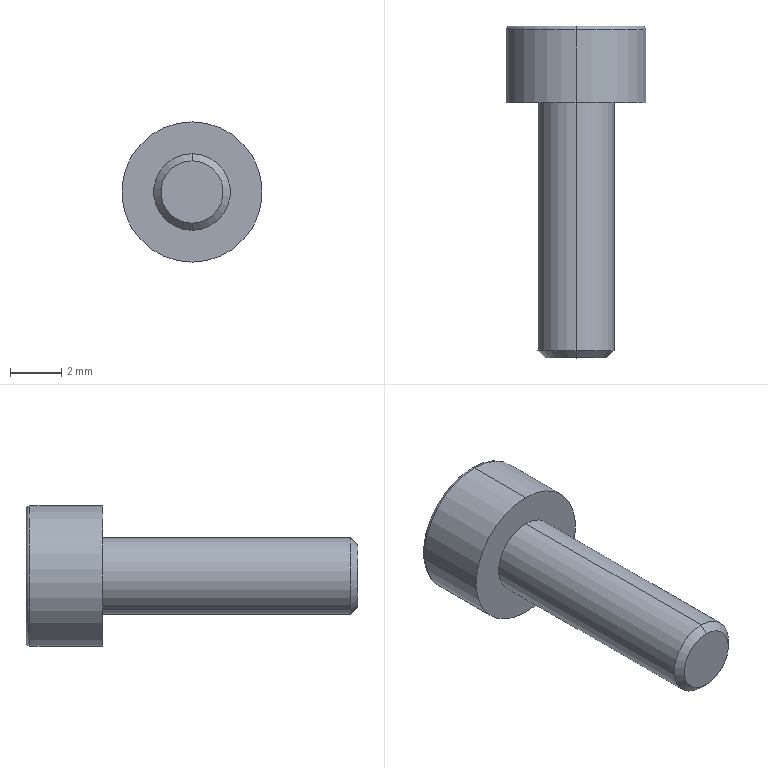Part | SolidWorks | features ICE 2, Chamfer 1, Extrusion 1, Fillet 1, RefAxis 1 | 1 solid | 18 faces | box 5.5 x 13 x 5.5 mm | volume 134.154 mm3 | plane 10 | cylinder 4 | cone 2 | torus 2 | commonest cylinder face diameters 3 x2 5.5 x2
STEP:
#1=CARTESIAN_POINT('',(0.,-10.,-1.22));
#2=VERTEX_POINT('',#1);
#3=CARTESIAN_POINT('',(0.,-10.,1.22));
#4=VERTEX_POINT('',#3);
#5=CARTESIAN_POINT('',(0.,-10.,0.));
#6=DIRECTION('',(0.,-1.,0.));
#7=DIRECTION('',(0.,0.,-1.));
#8=AXIS2_PLACEMENT_3D('',#5,#6,#7);
#9=CIRCLE('',#8,1.22);
#10=EDGE_CURVE('',#2,#4,#9,.T.);
#11=ORIENTED_EDGE('',*,*,#10,.F.);
#12=CARTESIAN_POINT('',(0.,-9.72,-1.5));
#13=VERTEX_POINT('',#12);
#14=CARTESIAN_POINT('',(0.,-10.,-1.22));
#15=DIRECTION('',(0.,0.7071,-0.7071));
#16=VECTOR('',#15,1000.);
#17=LINE('',#14,#16);
#18=EDGE_CURVE('',#2,#13,#17,.T.);
#19=ORIENTED_EDGE('',*,*,#18,.T.);
#20=CARTESIAN_POINT('',(0.,-9.72,1.5));
#21=VERTEX_POINT('',#20);
#22=CARTESIAN_POINT('',(0.,-9.72,0.));
#23=DIRECTION('',(0.,1.,0.));
#24=DIRECTION('',(0.,0.,-1.));
#25=AXIS2_PLACEMENT_3D('',#22,#23,#24);
#26=CIRCLE('',#25,1.5);
#27=EDGE_CURVE('',#21,#13,#26,.T.);
#28=ORIENTED_EDGE('',*,*,#27,.F.);
#29=CARTESIAN_POINT('',(0.,-10.,1.22));
#30=DIRECTION('',(0.,0.7071,0.7071));
#31=VECTOR('',#30,1000.);
#32=LINE('',#29,#31);
#33=EDGE_CURVE('',#4,#21,#32,.T.);
#34=ORIENTED_EDGE('',*,*,#33,.F.);
#35=EDGE_LOOP('',(#11,#19,#28,#34));
#36=FACE_OUTER_BOUND('',#35,.T.);
#37=CARTESIAN_POINT('',(0.,-10.,0.));
#38=DIRECTION('',(0.,1.,0.));
#39=DIRECTION('',(0.,0.,1.));
#40=AXIS2_PLACEMENT_3D('',#37,#38,#39);
#41=CONICAL_SURFACE('',#40,1.22,0.7854);
#42=ADVANCED_FACE('',(#36),#41,.T.);
#43=ORIENTED_EDGE('',*,*,#27,.T.);
#44=CARTESIAN_POINT('',(0.,0.,-1.5));
#45=VERTEX_POINT('',#44);
#46=CARTESIAN_POINT('',(0.,-10.,-1.5));
#47=DIRECTION('',(0.,1.,0.));
#48=VECTOR('',#47,1000.);
#49=LINE('',#46,#48);
#50=EDGE_CURVE('',#13,#45,#49,.T.);
#51=ORIENTED_EDGE('',*,*,#50,.T.);
#52=CARTESIAN_POINT('',(0.,0.,1.5));
#53=VERTEX_POINT('',#52);
#54=CARTESIAN_POINT('',(0.,0.,0.));
#55=DIRECTION('',(0.,-1.,0.));
#56=DIRECTION('',(0.,0.,1.));
#57=AXIS2_PLACEMENT_3D('',#54,#55,#56);
#58=CIRCLE('',#57,1.5);
#59=EDGE_CURVE('',#45,#53,#58,.T.);
#60=ORIENTED_EDGE('',*,*,#59,.T.);
#61=CARTESIAN_POINT('',(0.,-10.,1.5));
#62=DIRECTION('',(0.,1.,0.));
#63=VECTOR('',#62,1000.);
#64=LINE('',#61,#63);
#65=EDGE_CURVE('',#21,#53,#64,.T.);
#66=ORIENTED_EDGE('',*,*,#65,.F.);
#67=EDGE_LOOP('',(#43,#51,#60,#66));
#68=FACE_OUTER_BOUND('',#67,.T.);
#69=CARTESIAN_POINT('',(0.,-10.,0.));
#70=DIRECTION('',(0.,1.,0.));
#71=DIRECTION('',(0.,0.,1.));
#72=AXIS2_PLACEMENT_3D('',#69,#70,#71);
#73=CYLINDRICAL_SURFACE('',#72,1.5);
#74=ADVANCED_FACE('',(#68),#73,.T.);
#75=CARTESIAN_POINT('',(0.,2.85,-2.75));
#76=VERTEX_POINT('',#75);
#77=CARTESIAN_POINT('',(0.,2.85,2.75));
#78=VERTEX_POINT('',#77);
#79=CARTESIAN_POINT('',(0.,2.85,0.));
#80=DIRECTION('',(0.,-1.,0.));
#81=DIRECTION('',(0.,0.,1.));
#82=AXIS2_PLACEMENT_3D('',#79,#80,#81);
#83=CIRCLE('',#82,2.75);
#84=EDGE_CURVE('',#76,#78,#83,.T.);
#85=ORIENTED_EDGE('',*,*,#84,.F.);
#86=CARTESIAN_POINT('',(0.,3.,-2.6));
#87=VERTEX_POINT('',#86);
#88=CARTESIAN_POINT('',(0.,2.85,-2.6));
#89=DIRECTION('',(1.,0.,0.));
#90=DIRECTION('',(0.,0.,-1.));
#91=AXIS2_PLACEMENT_3D('',#88,#89,#90);
#92=CIRCLE('',#91,0.15);
#93=EDGE_CURVE('',#76,#87,#92,.T.);
#94=ORIENTED_EDGE('',*,*,#93,.T.);
#95=CARTESIAN_POINT('',(0.,3.,2.6));
#96=VERTEX_POINT('',#95);
#97=CARTESIAN_POINT('',(0.,3.,0.));
#98=DIRECTION('',(0.,1.,0.));
#99=DIRECTION('',(0.,0.,1.));
#100=AXIS2_PLACEMENT_3D('',#97,#98,#99);
#101=CIRCLE('',#100,2.6);
#102=EDGE_CURVE('',#96,#87,#101,.T.);
#103=ORIENTED_EDGE('',*,*,#102,.F.);
#104=CARTESIAN_POINT('',(0.,2.85,2.6));
#105=DIRECTION('',(-1.,0.,0.));
#106=DIRECTION('',(0.,0.,1.));
#107=AXIS2_PLACEMENT_3D('',#104,#105,#106);
#108=CIRCLE('',#107,0.15);
#109=EDGE_CURVE('',#78,#96,#108,.T.);
#110=ORIENTED_EDGE('',*,*,#109,.F.);
#111=EDGE_LOOP('',(#85,#94,#103,#110));
#112=FACE_OUTER_BOUND('',#111,.T.);
#113=CARTESIAN_POINT('',(0.,2.85,0.));
#114=DIRECTION('',(0.,1.,0.));
#115=DIRECTION('',(0.,0.,1.));
#116=AXIS2_PLACEMENT_3D('',#113,#114,#115);
#117=TOROIDAL_SURFACE('',#116,2.6,0.15);
#118=ADVANCED_FACE('',(#112),#117,.T.);
#119=ORIENTED_EDGE('',*,*,#84,.T.);
#120=CARTESIAN_POINT('',(0.,0.,2.75));
#121=VERTEX_POINT('',#120);
#122=CARTESIAN_POINT('',(0.,3.,2.75));
#123=DIRECTION('',(0.,-1.,0.));
#124=VECTOR('',#123,1000.);
#125=LINE('',#122,#124);
#126=EDGE_CURVE('',#78,#121,#125,.T.);
#127=ORIENTED_EDGE('',*,*,#126,.T.);
#128=CARTESIAN_POINT('',(0.,0.,-2.75));
#129=VERTEX_POINT('',#128);
#130=CARTESIAN_POINT('',(0.,0.,0.));
#131=DIRECTION('',(0.,1.,0.));
#132=DIRECTION('',(0.,0.,1.));
#133=AXIS2_PLACEMENT_3D('',#130,#131,#132);
#134=CIRCLE('',#133,2.75);
#135=EDGE_CURVE('',#121,#129,#134,.T.);
#136=ORIENTED_EDGE('',*,*,#135,.T.);
#137=CARTESIAN_POINT('',(0.,3.,-2.75));
#138=DIRECTION('',(0.,-1.,0.));
#139=VECTOR('',#138,1000.);
#140=LINE('',#137,#139);
#141=EDGE_CURVE('',#76,#129,#140,.T.);
#142=ORIENTED_EDGE('',*,*,#141,.F.);
#143=EDGE_LOOP('',(#119,#127,#136,#142));
#144=FACE_OUTER_BOUND('',#143,.T.);
#145=CARTESIAN_POINT('',(0.,3.,0.));
#146=DIRECTION('',(0.,-1.,0.));
#147=DIRECTION('',(0.,0.,-1.));
#148=AXIS2_PLACEMENT_3D('',#145,#146,#147);
#149=CYLINDRICAL_SURFACE('',#148,2.75);
#150=ADVANCED_FACE('',(#144),#149,.T.);
#151=CARTESIAN_POINT('',(0.,0.,0.));
#152=DIRECTION('',(0.,1.,0.));
#153=DIRECTION('',(0.,0.,1.));
#154=AXIS2_PLACEMENT_3D('',#151,#152,#153);
#155=CIRCLE('',#154,2.75);
#156=EDGE_CURVE('',#129,#121,#155,.T.);
#157=ORIENTED_EDGE('',*,*,#156,.F.);
#158=ORIENTED_EDGE('',*,*,#135,.F.);
#159=EDGE_LOOP('',(#157,#158));
#160=FACE_OUTER_BOUND('',#159,.T.);
#161=CARTESIAN_POINT('',(0.,0.,0.));
#162=DIRECTION('',(0.,-1.,0.));
#163=DIRECTION('',(0.,0.,1.));
#164=AXIS2_PLACEMENT_3D('',#161,#162,#163);
#165=CIRCLE('',#164,1.5);
#166=EDGE_CURVE('',#53,#45,#165,.T.);
#167=ORIENTED_EDGE('',*,*,#166,.F.);
#168=ORIENTED_EDGE('',*,*,#59,.F.);
#169=EDGE_LOOP('',(#167,#168));
#170=FACE_BOUND('',#169,.T.);
#171=CARTESIAN_POINT('',(0.,0.,0.));
#172=DIRECTION('',(0.,1.,0.));
#173=DIRECTION('',(0.,0.,1.));
#174=AXIS2_PLACEMENT_3D('',#171,#172,#173);
#175=PLANE('',#174);
#176=ADVANCED_FACE('',(#160,#170),#175,.F.);
#177=ORIENTED_EDGE('',*,*,#126,.F.);
#178=CARTESIAN_POINT('',(0.,2.85,0.));
#179=DIRECTION('',(0.,-1.,0.));
#180=DIRECTION('',(0.,0.,1.));
#181=AXIS2_PLACEMENT_3D('',#178,#179,#180);
#182=CIRCLE('',#181,2.75);
#183=EDGE_CURVE('',#78,#76,#182,.T.);
#184=ORIENTED_EDGE('',*,*,#183,.T.);
#185=ORIENTED_EDGE('',*,*,#141,.T.);
#186=ORIENTED_EDGE('',*,*,#156,.T.);
#187=EDGE_LOOP('',(#177,#184,#185,#186));
#188=FACE_OUTER_BOUND('',#187,.T.);
#189=CARTESIAN_POINT('',(0.,3.,0.));
#190=DIRECTION('',(0.,-1.,0.));
#191=DIRECTION('',(0.,0.,-1.));
#192=AXIS2_PLACEMENT_3D('',#189,#190,#191);
#193=CYLINDRICAL_SURFACE('',#192,2.75);
#194=ADVANCED_FACE('',(#188),#193,.T.);
#195=ORIENTED_EDGE('',*,*,#102,.T.);
#196=CARTESIAN_POINT('',(0.,3.,0.));
#197=DIRECTION('',(0.,1.,0.));
#198=DIRECTION('',(0.,0.,1.));
#199=AXIS2_PLACEMENT_3D('',#196,#197,#198);
#200=CIRCLE('',#199,2.6);
#201=EDGE_CURVE('',#87,#96,#200,.T.);
#202=ORIENTED_EDGE('',*,*,#201,.T.);
#203=EDGE_LOOP('',(#195,#202));
#204=FACE_OUTER_BOUND('',#203,.T.);
#205=CARTESIAN_POINT('',(0.739,3.,1.28));
#206=VERTEX_POINT('',#205);
#207=CARTESIAN_POINT('',(1.478,3.,0.));
#208=VERTEX_POINT('',#207);
#209=CARTESIAN_POINT('',(0.739,3.,1.28));
#210=DIRECTION('',(0.5,0.,-0.866));
#211=VECTOR('',#210,1000.);
#212=LINE('',#209,#211);
#213=EDGE_CURVE('',#206,#208,#212,.T.);
#214=ORIENTED_EDGE('',*,*,#213,.F.);
#215=CARTESIAN_POINT('',(-0.739,3.,1.28));
#216=VERTEX_POINT('',#215);
#217=CARTESIAN_POINT('',(-0.739,3.,1.28));
#218=DIRECTION('',(1.,0.,0.));
#219=VECTOR('',#218,1000.);
#220=LINE('',#217,#219);
#221=EDGE_CURVE('',#216,#206,#220,.T.);
#222=ORIENTED_EDGE('',*,*,#221,.F.);
#223=CARTESIAN_POINT('',(-1.478,3.,0.));
#224=VERTEX_POINT('',#223);
#225=CARTESIAN_POINT('',(-1.478,3.,0.));
#226=DIRECTION('',(0.5,0.,0.866));
#227=VECTOR('',#226,1000.);
#228=LINE('',#225,#227);
#229=EDGE_CURVE('',#224,#216,#228,.T.);
#230=ORIENTED_EDGE('',*,*,#229,.F.);
#231=CARTESIAN_POINT('',(-0.739,3.,-1.28));
#232=VERTEX_POINT('',#231);
#233=CARTESIAN_POINT('',(-0.739,3.,-1.28));
#234=DIRECTION('',(-0.5,0.,0.866));
#235=VECTOR('',#234,1000.);
#236=LINE('',#233,#235);
#237=EDGE_CURVE('',#232,#224,#236,.T.);
#238=ORIENTED_EDGE('',*,*,#237,.F.);
#239=CARTESIAN_POINT('',(0.739,3.,-1.28));
#240=VERTEX_POINT('',#239);
#241=CARTESIAN_POINT('',(0.739,3.,-1.28));
#242=DIRECTION('',(-1.,0.,0.));
#243=VECTOR('',#242,1000.);
#244=LINE('',#241,#243);
#245=EDGE_CURVE('',#240,#232,#244,.T.);
#246=ORIENTED_EDGE('',*,*,#245,.F.);
#247=CARTESIAN_POINT('',(1.478,3.,0.));
#248=DIRECTION('',(-0.5,0.,-0.866));
#249=VECTOR('',#248,1000.);
#250=LINE('',#247,#249);
#251=EDGE_CURVE('',#208,#240,#250,.T.);
#252=ORIENTED_EDGE('',*,*,#251,.F.);
#253=EDGE_LOOP('',(#214,#222,#230,#238,#246,#252));
#254=FACE_BOUND('',#253,.T.);
#255=CARTESIAN_POINT('',(0.,3.,0.));
#256=DIRECTION('',(0.,1.,0.));
#257=DIRECTION('',(0.,0.,1.));
#258=AXIS2_PLACEMENT_3D('',#255,#256,#257);
#259=PLANE('',#258);
#260=ADVANCED_FACE('',(#204,#254),#259,.T.);
#261=ORIENTED_EDGE('',*,*,#213,.T.);
#262=CARTESIAN_POINT('',(1.478,1.7,0.));
#263=VERTEX_POINT('',#262);
#264=CARTESIAN_POINT('',(1.478,1.7,0.));
#265=DIRECTION('',(0.,1.,0.));
#266=VECTOR('',#265,1000.);
#267=LINE('',#264,#266);
#268=EDGE_CURVE('',#263,#208,#267,.T.);
#269=ORIENTED_EDGE('',*,*,#268,.F.);
#270=CARTESIAN_POINT('',(0.739,1.7,1.28));
#271=VERTEX_POINT('',#270);
#272=CARTESIAN_POINT('',(0.739,1.7,1.28));
#273=DIRECTION('',(0.5,0.,-0.866));
#274=VECTOR('',#273,1000.);
#275=LINE('',#272,#274);
#276=EDGE_CURVE('',#271,#263,#275,.T.);
#277=ORIENTED_EDGE('',*,*,#276,.F.);
#278=CARTESIAN_POINT('',(0.739,1.7,1.28));
#279=DIRECTION('',(0.,1.,0.));
#280=VECTOR('',#279,1000.);
#281=LINE('',#278,#280);
#282=EDGE_CURVE('',#271,#206,#281,.T.);
#283=ORIENTED_EDGE('',*,*,#282,.T.);
#284=EDGE_LOOP('',(#261,#269,#277,#283));
#285=FACE_OUTER_BOUND('',#284,.T.);
#286=CARTESIAN_POINT('',(0.739,1.7,1.28));
#287=DIRECTION('',(0.866,0.,0.5));
#288=DIRECTION('',(0.5,0.,-0.866));
#289=AXIS2_PLACEMENT_3D('',#286,#287,#288);
#290=PLANE('',#289);
#291=ADVANCED_FACE('',(#285),#290,.F.);
#292=ORIENTED_EDGE('',*,*,#221,.T.);
#293=ORIENTED_EDGE('',*,*,#282,.F.);
#294=CARTESIAN_POINT('',(-0.739,1.7,1.28));
#295=VERTEX_POINT('',#294);
#296=CARTESIAN_POINT('',(-0.739,1.7,1.28));
#297=DIRECTION('',(1.,0.,0.));
#298=VECTOR('',#297,1000.);
#299=LINE('',#296,#298);
#300=EDGE_CURVE('',#295,#271,#299,.T.);
#301=ORIENTED_EDGE('',*,*,#300,.F.);
#302=CARTESIAN_POINT('',(-0.739,1.7,1.28));
#303=DIRECTION('',(0.,1.,0.));
#304=VECTOR('',#303,1000.);
#305=LINE('',#302,#304);
#306=EDGE_CURVE('',#295,#216,#305,.T.);
#307=ORIENTED_EDGE('',*,*,#306,.T.);
#308=EDGE_LOOP('',(#292,#293,#301,#307));
#309=FACE_OUTER_BOUND('',#308,.T.);
#310=CARTESIAN_POINT('',(-0.739,1.7,1.28));
#311=DIRECTION('',(0.,0.,1.));
#312=DIRECTION('',(1.,0.,0.));
#313=AXIS2_PLACEMENT_3D('',#310,#311,#312);
#314=PLANE('',#313);
#315=ADVANCED_FACE('',(#309),#314,.F.);
#316=ORIENTED_EDGE('',*,*,#229,.T.);
#317=ORIENTED_EDGE('',*,*,#306,.F.);
#318=CARTESIAN_POINT('',(-1.478,1.7,0.));
#319=VERTEX_POINT('',#318);
#320=CARTESIAN_POINT('',(-1.478,1.7,0.));
#321=DIRECTION('',(0.5,0.,0.866));
#322=VECTOR('',#321,1000.);
#323=LINE('',#320,#322);
#324=EDGE_CURVE('',#319,#295,#323,.T.);
#325=ORIENTED_EDGE('',*,*,#324,.F.);
#326=CARTESIAN_POINT('',(-1.478,1.7,0.));
#327=DIRECTION('',(0.,1.,0.));
#328=VECTOR('',#327,1000.);
#329=LINE('',#326,#328);
#330=EDGE_CURVE('',#319,#224,#329,.T.);
#331=ORIENTED_EDGE('',*,*,#330,.T.);
#332=EDGE_LOOP('',(#316,#317,#325,#331));
#333=FACE_OUTER_BOUND('',#332,.T.);
#334=CARTESIAN_POINT('',(-1.478,1.7,0.));
#335=DIRECTION('',(-0.866,0.,0.5));
#336=DIRECTION('',(0.5,0.,0.866));
#337=AXIS2_PLACEMENT_3D('',#334,#335,#336);
#338=PLANE('',#337);
#339=ADVANCED_FACE('',(#333),#338,.F.);
#340=ORIENTED_EDGE('',*,*,#237,.T.);
#341=ORIENTED_EDGE('',*,*,#330,.F.);
#342=CARTESIAN_POINT('',(-0.739,1.7,-1.28));
#343=VERTEX_POINT('',#342);
#344=CARTESIAN_POINT('',(-0.739,1.7,-1.28));
#345=DIRECTION('',(-0.5,0.,0.866));
#346=VECTOR('',#345,1000.);
#347=LINE('',#344,#346);
#348=EDGE_CURVE('',#343,#319,#347,.T.);
#349=ORIENTED_EDGE('',*,*,#348,.F.);
#350=CARTESIAN_POINT('',(-0.739,1.7,-1.28));
#351=DIRECTION('',(0.,1.,0.));
#352=VECTOR('',#351,1000.);
#353=LINE('',#350,#352);
#354=EDGE_CURVE('',#343,#232,#353,.T.);
#355=ORIENTED_EDGE('',*,*,#354,.T.);
#356=EDGE_LOOP('',(#340,#341,#349,#355));
#357=FACE_OUTER_BOUND('',#356,.T.);
#358=CARTESIAN_POINT('',(-0.739,1.7,-1.28));
#359=DIRECTION('',(-0.866,0.,-0.5));
#360=DIRECTION('',(-0.5,0.,0.866));
#361=AXIS2_PLACEMENT_3D('',#358,#359,#360);
#362=PLANE('',#361);
#363=ADVANCED_FACE('',(#357),#362,.F.);
#364=ORIENTED_EDGE('',*,*,#245,.T.);
#365=ORIENTED_EDGE('',*,*,#354,.F.);
#366=CARTESIAN_POINT('',(0.739,1.7,-1.28));
#367=VERTEX_POINT('',#366);
#368=CARTESIAN_POINT('',(0.739,1.7,-1.28));
#369=DIRECTION('',(-1.,0.,0.));
#370=VECTOR('',#369,1000.);
#371=LINE('',#368,#370);
#372=EDGE_CURVE('',#367,#343,#371,.T.);
#373=ORIENTED_EDGE('',*,*,#372,.F.);
#374=CARTESIAN_POINT('',(0.739,1.7,-1.28));
#375=DIRECTION('',(0.,1.,0.));
#376=VECTOR('',#375,1000.);
#377=LINE('',#374,#376);
#378=EDGE_CURVE('',#367,#240,#377,.T.);
#379=ORIENTED_EDGE('',*,*,#378,.T.);
#380=EDGE_LOOP('',(#364,#365,#373,#379));
#381=FACE_OUTER_BOUND('',#380,.T.);
#382=CARTESIAN_POINT('',(0.739,1.7,-1.28));
#383=DIRECTION('',(0.,0.,-1.));
#384=DIRECTION('',(-1.,0.,0.));
#385=AXIS2_PLACEMENT_3D('',#382,#383,#384);
#386=PLANE('',#385);
#387=ADVANCED_FACE('',(#381),#386,.F.);
#388=ORIENTED_EDGE('',*,*,#251,.T.);
#389=ORIENTED_EDGE('',*,*,#378,.F.);
#390=CARTESIAN_POINT('',(1.478,1.7,0.));
#391=DIRECTION('',(-0.5,0.,-0.866));
#392=VECTOR('',#391,1000.);
#393=LINE('',#390,#392);
#394=EDGE_CURVE('',#263,#367,#393,.T.);
#395=ORIENTED_EDGE('',*,*,#394,.F.);
#396=ORIENTED_EDGE('',*,*,#268,.T.);
#397=EDGE_LOOP('',(#388,#389,#395,#396));
#398=FACE_OUTER_BOUND('',#397,.T.);
#399=CARTESIAN_POINT('',(1.478,1.7,0.));
#400=DIRECTION('',(0.866,0.,-0.5));
#401=DIRECTION('',(-0.5,0.,-0.866));
#402=AXIS2_PLACEMENT_3D('',#399,#400,#401);
#403=PLANE('',#402);
#404=ADVANCED_FACE('',(#398),#403,.F.);
#405=ORIENTED_EDGE('',*,*,#276,.T.);
#406=ORIENTED_EDGE('',*,*,#394,.T.);
#407=ORIENTED_EDGE('',*,*,#372,.T.);
#408=ORIENTED_EDGE('',*,*,#348,.T.);
#409=ORIENTED_EDGE('',*,*,#324,.T.);
#410=ORIENTED_EDGE('',*,*,#300,.T.);
#411=EDGE_LOOP('',(#405,#406,#407,#408,#409,#410));
#412=FACE_OUTER_BOUND('',#411,.T.);
#413=CARTESIAN_POINT('',(0.,1.7,0.));
#414=DIRECTION('',(0.,1.,0.));
#415=DIRECTION('',(0.,0.,1.));
#416=AXIS2_PLACEMENT_3D('',#413,#414,#415);
#417=PLANE('',#416);
#418=ADVANCED_FACE('',(#412),#417,.T.);
#419=ORIENTED_EDGE('',*,*,#93,.F.);
#420=ORIENTED_EDGE('',*,*,#183,.F.);
#421=ORIENTED_EDGE('',*,*,#109,.T.);
#422=ORIENTED_EDGE('',*,*,#201,.F.);
#423=EDGE_LOOP('',(#419,#420,#421,#422));
#424=FACE_OUTER_BOUND('',#423,.T.);
#425=CARTESIAN_POINT('',(0.,2.85,0.));
#426=DIRECTION('',(0.,1.,0.));
#427=DIRECTION('',(0.,0.,1.));
#428=AXIS2_PLACEMENT_3D('',#425,#426,#427);
#429=TOROIDAL_SURFACE('',#428,2.6,0.15);
#430=ADVANCED_FACE('',(#424),#429,.T.);
#431=ORIENTED_EDGE('',*,*,#50,.F.);
#432=CARTESIAN_POINT('',(0.,-9.72,0.));
#433=DIRECTION('',(0.,1.,0.));
#434=DIRECTION('',(0.,0.,-1.));
#435=AXIS2_PLACEMENT_3D('',#432,#433,#434);
#436=CIRCLE('',#435,1.5);
#437=EDGE_CURVE('',#13,#21,#436,.T.);
#438=ORIENTED_EDGE('',*,*,#437,.T.);
#439=ORIENTED_EDGE('',*,*,#65,.T.);
#440=ORIENTED_EDGE('',*,*,#166,.T.);
#441=EDGE_LOOP('',(#431,#438,#439,#440));
#442=FACE_OUTER_BOUND('',#441,.T.);
#443=CARTESIAN_POINT('',(0.,-10.,0.));
#444=DIRECTION('',(0.,1.,0.));
#445=DIRECTION('',(0.,0.,1.));
#446=AXIS2_PLACEMENT_3D('',#443,#444,#445);
#447=CYLINDRICAL_SURFACE('',#446,1.5);
#448=ADVANCED_FACE('',(#442),#447,.T.);
#449=CARTESIAN_POINT('',(0.,-10.,0.));
#450=DIRECTION('',(0.,-1.,0.));
#451=DIRECTION('',(0.,0.,-1.));
#452=AXIS2_PLACEMENT_3D('',#449,#450,#451);
#453=CIRCLE('',#452,1.22);
#454=EDGE_CURVE('',#4,#2,#453,.T.);
#455=ORIENTED_EDGE('',*,*,#454,.T.);
#456=ORIENTED_EDGE('',*,*,#10,.T.);
#457=EDGE_LOOP('',(#455,#456));
#458=FACE_OUTER_BOUND('',#457,.T.);
#459=CARTESIAN_POINT('',(0.,-10.,0.));
#460=DIRECTION('',(0.,-1.,0.));
#461=DIRECTION('',(0.,0.,-1.));
#462=AXIS2_PLACEMENT_3D('',#459,#460,#461);
#463=PLANE('',#462);
#464=ADVANCED_FACE('',(#458),#463,.T.);
#465=ORIENTED_EDGE('',*,*,#18,.F.);
#466=ORIENTED_EDGE('',*,*,#454,.F.);
#467=ORIENTED_EDGE('',*,*,#33,.T.);
#468=ORIENTED_EDGE('',*,*,#437,.F.);
#469=EDGE_LOOP('',(#465,#466,#467,#468));
#470=FACE_OUTER_BOUND('',#469,.T.);
#471=CARTESIAN_POINT('',(0.,-10.,0.));
#472=DIRECTION('',(0.,1.,0.));
#473=DIRECTION('',(0.,0.,1.));
#474=AXIS2_PLACEMENT_3D('',#471,#472,#473);
#475=CONICAL_SURFACE('',#474,1.22,0.7854);
#476=ADVANCED_FACE('',(#470),#475,.T.);
#477=CLOSED_SHELL('',(#42,#74,#118,#150,#176,#194,#260,#291,#315,#339,#363,#387,#404,#418,#430,#448,#464,#476));
#478=MANIFOLD_SOLID_BREP('',#477);
#479=CARTESIAN_POINT('',(0.,0.,0.));
#480=DIRECTION('',(0.,0.,1.));
#481=DIRECTION('',(1.,0.,0.));
#482=AXIS2_PLACEMENT_3D('',#479,#480,#481);
#483=(LENGTH_UNIT()NAMED_UNIT(*)SI_UNIT(.MILLI.,.METRE.));
#484=UNCERTAINTY_MEASURE_WITH_UNIT(LENGTH_MEASURE(0.00001),#483,'','');
#485=(NAMED_UNIT(*)PLANE_ANGLE_UNIT()SI_UNIT($,.RADIAN.));
#486=(NAMED_UNIT(*)SI_UNIT($,.STERADIAN.)SOLID_ANGLE_UNIT());
#487=(GEOMETRIC_REPRESENTATION_CONTEXT(3)GLOBAL_UNCERTAINTY_ASSIGNED_CONTEXT((#484))GLOBAL_UNIT_ASSIGNED_CONTEXT((#483,#485,#486))REPRESENTATION_CONTEXT('',''));
#488=ADVANCED_BREP_SHAPE_REPRESENTATION('',(#478,#482),#487);